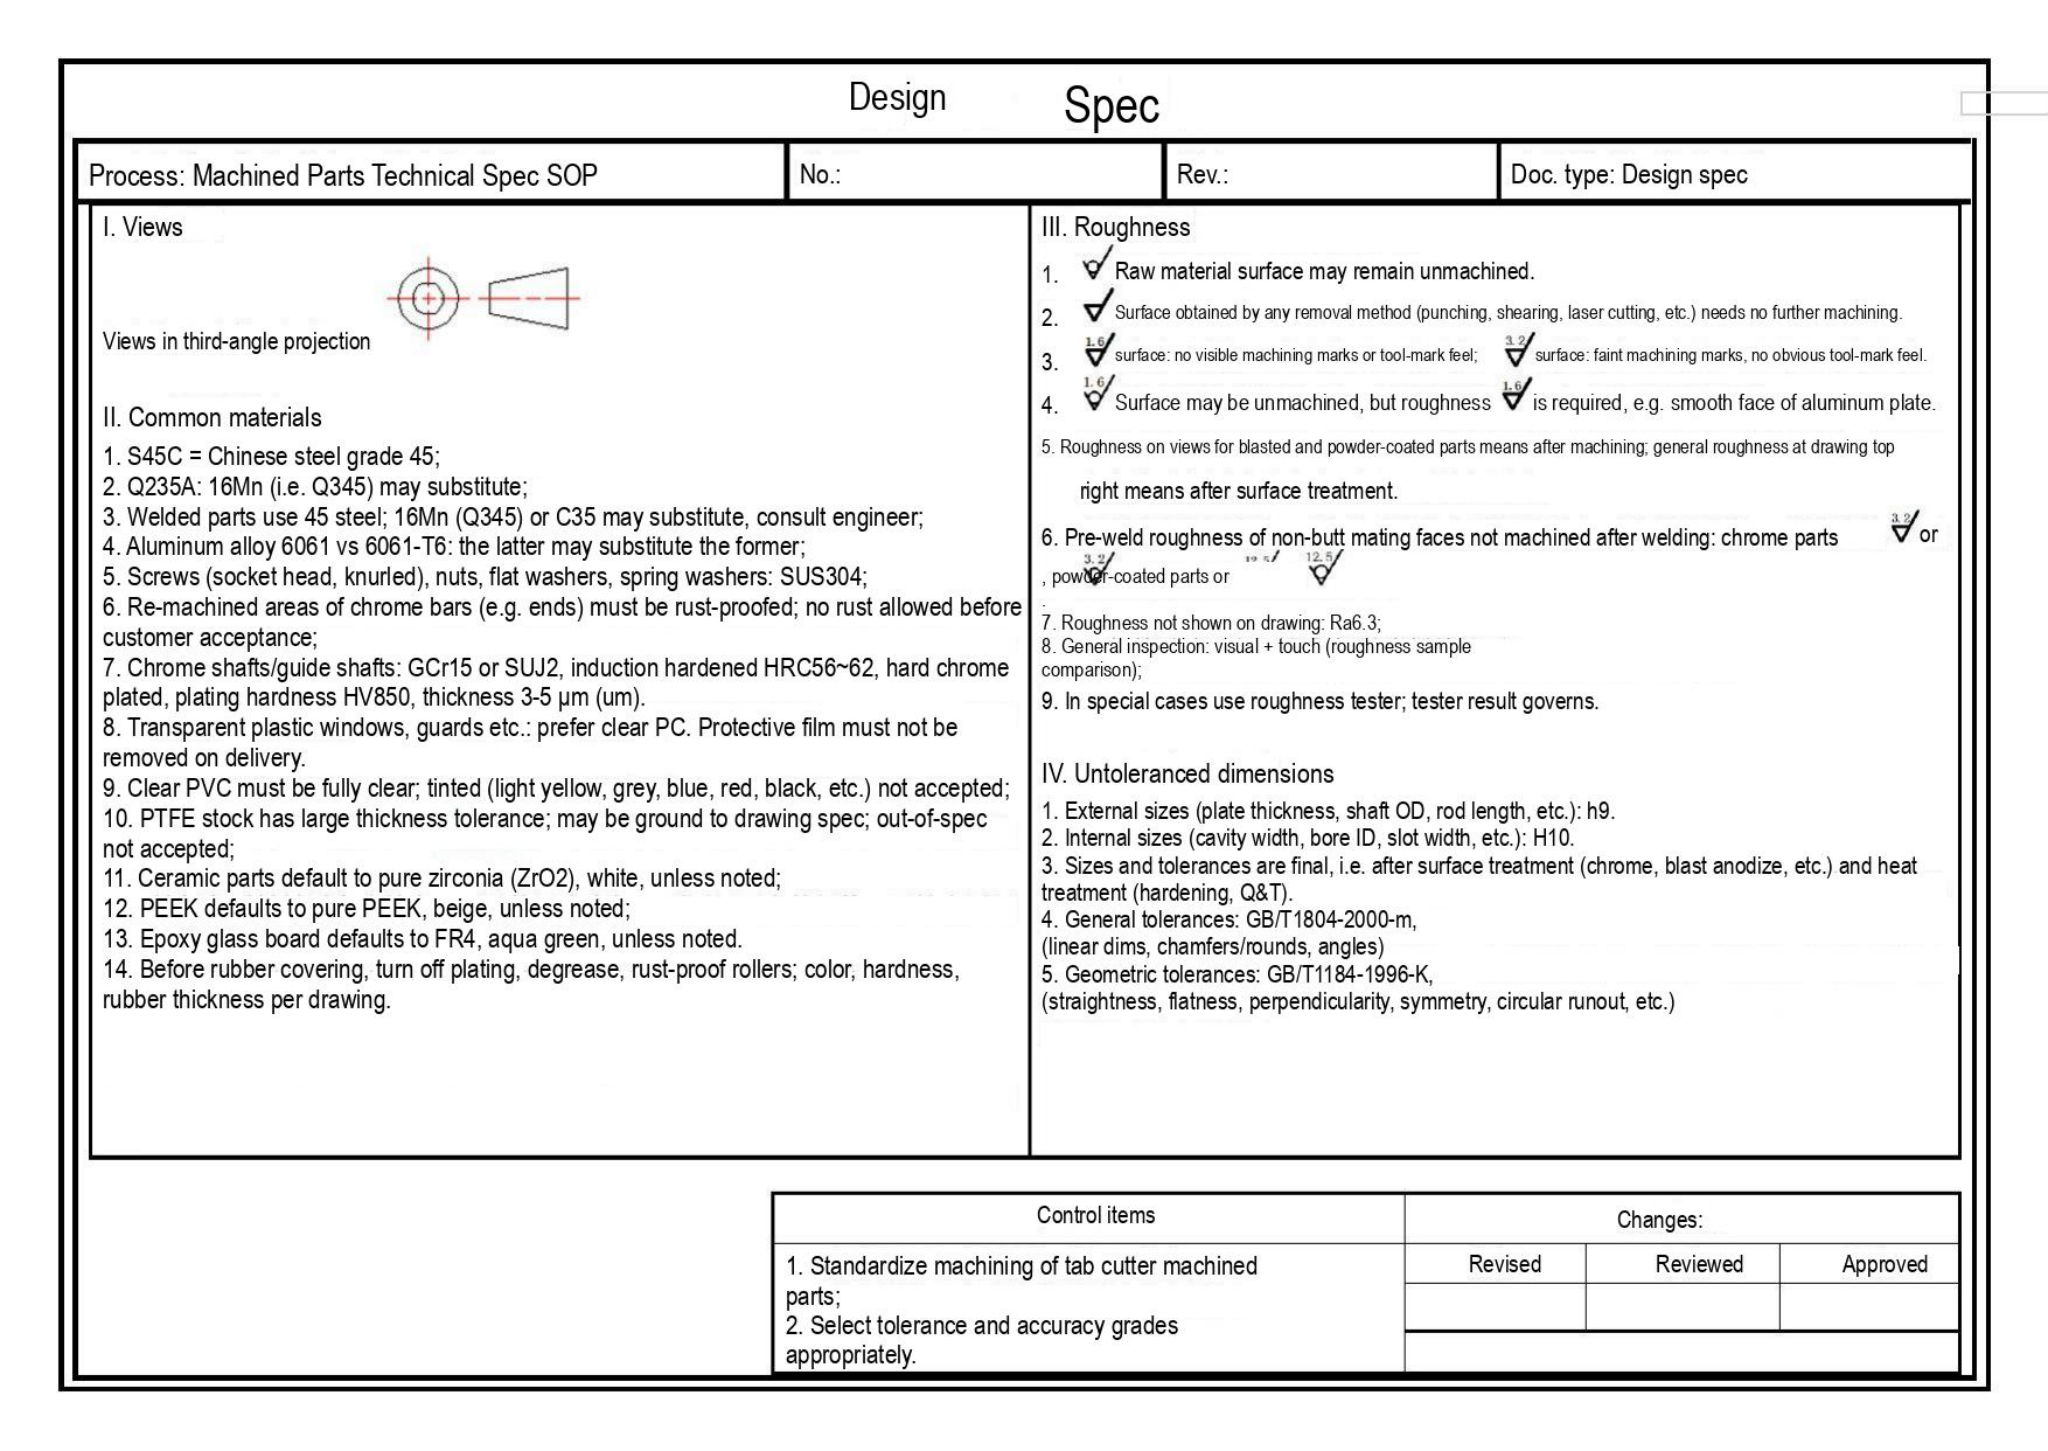Design Spec

| Process: Machined Parts Technical Spec SOP | No.: | Rev.: | Doc. type: Design spec |
|---|---|---|---|

I. Views

Views in third-angle projection

II. Common materials

1. S45C = Chinese steel grade 45;
2. Q235A: 16Mn (i.e. Q345) may substitute;
3. Welded parts use 45 steel; 16Mn (Q345) or C35 may substitute, consult engineer;
4. Aluminum alloy 6061 vs 6061-T6: the latter may substitute the former;
5. Screws (socket head, knurled), nuts, flat washers, spring washers: SUS304;
6. Re-machined areas of chrome bars (e.g. ends) must be rust-proofed; no rust allowed before customer acceptance;
7. Chrome shafts/guide shafts: GCr15 or SUJ2, induction hardened HRC56~62, hard chrome plated, plating hardness HV850, thickness 3-5 μm (um).
8. Transparent plastic windows, guards etc.: prefer clear PC. Protective film must not be removed on delivery.
9. Clear PVC must be fully clear; tinted (light yellow, grey, blue, red, black, etc.) not accepted;
10. PTFE stock has large thickness tolerance; may be ground to drawing spec; out-of-spec not accepted;
11. Ceramic parts default to pure zirconia (ZrO2), white, unless noted;
12. PEEK defaults to pure PEEK, beige, unless noted;
13. Epoxy glass board defaults to FR4, aqua green, unless noted.
14. Before rubber covering, turn off plating, degrease, rust-proof rollers; color, hardness, rubber thickness per drawing.

III. Roughness

1. Raw material surface may remain unmachined.
2. Surface obtained by any removal method (punching, shearing, laser cutting, etc.) needs no further machining.
3. 1.6 surface: no visible machining marks or tool-mark feel; 3.2 surface: faint machining marks, no obvious tool-mark feel.
4. 1.6 Surface may be unmachined, but roughness 1.6 is required, e.g. smooth face of aluminum plate.
5. Roughness on views for blasted and powder-coated parts means after machining; general roughness at drawing top right means after surface treatment.
6. Pre-weld roughness of non-butt mating faces not machined after welding: chrome parts 3.2 or 3.2, powder-coated parts or 12.5
7. Roughness not shown on drawing: Ra6.3;
8. General inspection: visual + touch (roughness sample comparison);
9. In special cases use roughness tester; tester result governs.

IV. Untoleranced dimensions

1. External sizes (plate thickness, shaft OD, rod length, etc.): h9.
2. Internal sizes (cavity width, bore ID, slot width, etc.): H10.
3. Sizes and tolerances are final, i.e. after surface treatment (chrome, blast anodize, etc.) and heat treatment (hardening, Q&T).
4. General tolerances: GB/T1804-2000-m, (linear dims, chamfers/rounds, angles)
5. Geometric tolerances: GB/T1184-1996-K, (straightness, flatness, perpendicularity, symmetry, circular runout, etc.)

| Control items | Changes: | | |
|---|---|---|---|
| 1. Standardize machining of tab cutter machined parts;<br>2. Select tolerance and accuracy grades appropriately. | Revised | Reviewed | Approved |
| | | | |
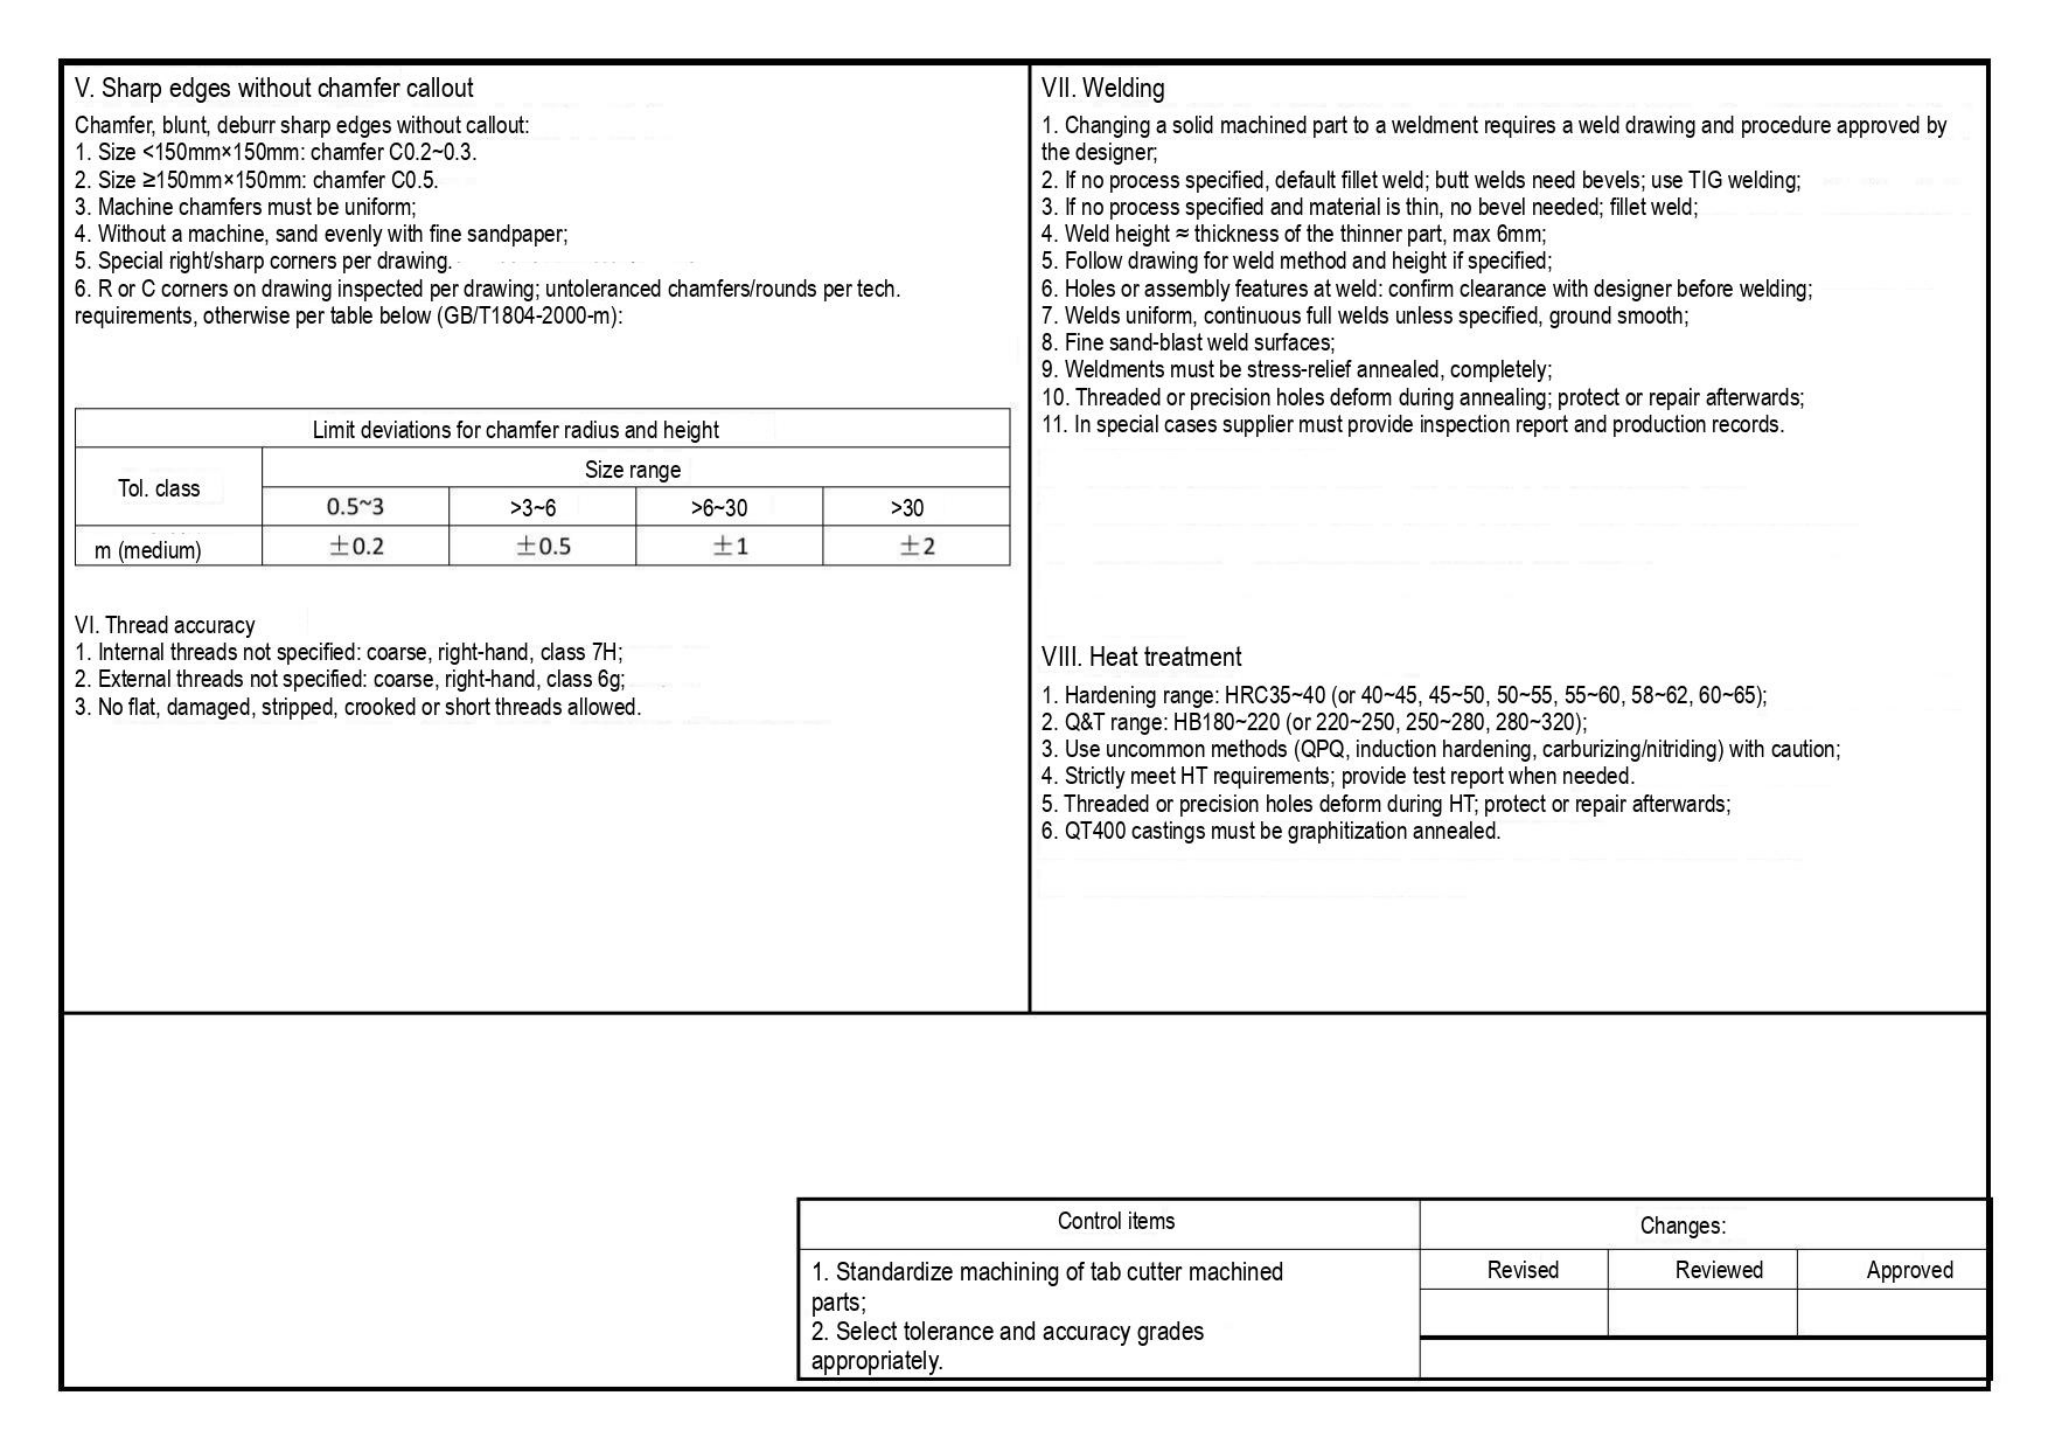V. Sharp edges without chamfer callout

Chamfer, blunt, deburr sharp edges without callout:
1. Size <150mm×150mm: chamfer C0.2~0.3.
2. Size ≥150mm×150mm: chamfer C0.5.
3. Machine chamfers must be uniform;
4. Without a machine, sand evenly with fine sandpaper;
5. Special right/sharp corners per drawing.
6. R or C corners on drawing inspected per drawing; untoleranced chamfers/rounds per tech. requirements, otherwise per table below (GB/T1804-2000-m):

Limit deviations for chamfer radius and height

| Tol. class | Size range | | | |
|---|---|---|---|---|
| | 0.5~3 | >3~6 | >6~30 | >30 |
| m (medium) | ±0.2 | ±0.5 | ±1 | ±2 |

VI. Thread accuracy
1. Internal threads not specified: coarse, right-hand, class 7H;
2. External threads not specified: coarse, right-hand, class 6g;
3. No flat, damaged, stripped, crooked or short threads allowed.

VII. Welding
1. Changing a solid machined part to a weldment requires a weld drawing and procedure approved by the designer;
2. If no process specified, default fillet weld; butt welds need bevels; use TIG welding;
3. If no process specified and material is thin, no bevel needed; fillet weld;
4. Weld height ≈ thickness of the thinner part, max 6mm;
5. Follow drawing for weld method and height if specified;
6. Holes or assembly features at weld: confirm clearance with designer before welding;
7. Welds uniform, continuous full welds unless specified, ground smooth;
8. Fine sand-blast weld surfaces;
9. Weldments must be stress-relief annealed, completely;
10. Threaded or precision holes deform during annealing; protect or repair afterwards;
11. In special cases supplier must provide inspection report and production records.

VIII. Heat treatment
1. Hardening range: HRC35~40 (or 40~45, 45~50, 50~55, 55~60, 58~62, 60~65);
2. Q&T range: HB180~220 (or 220~250, 250~280, 280~320);
3. Use uncommon methods (QPQ, induction hardening, carburizing/nitriding) with caution;
4. Strictly meet HT requirements; provide test report when needed.
5. Threaded or precision holes deform during HT; protect or repair afterwards;
6. QT400 castings must be graphitization annealed.

| Control items | Changes: | | |
|---|---|---|---|
| 1. Standardize machining of tab cutter machined parts;<br>2. Select tolerance and accuracy grades appropriately. | Revised | Reviewed | Approved |
| | | | |
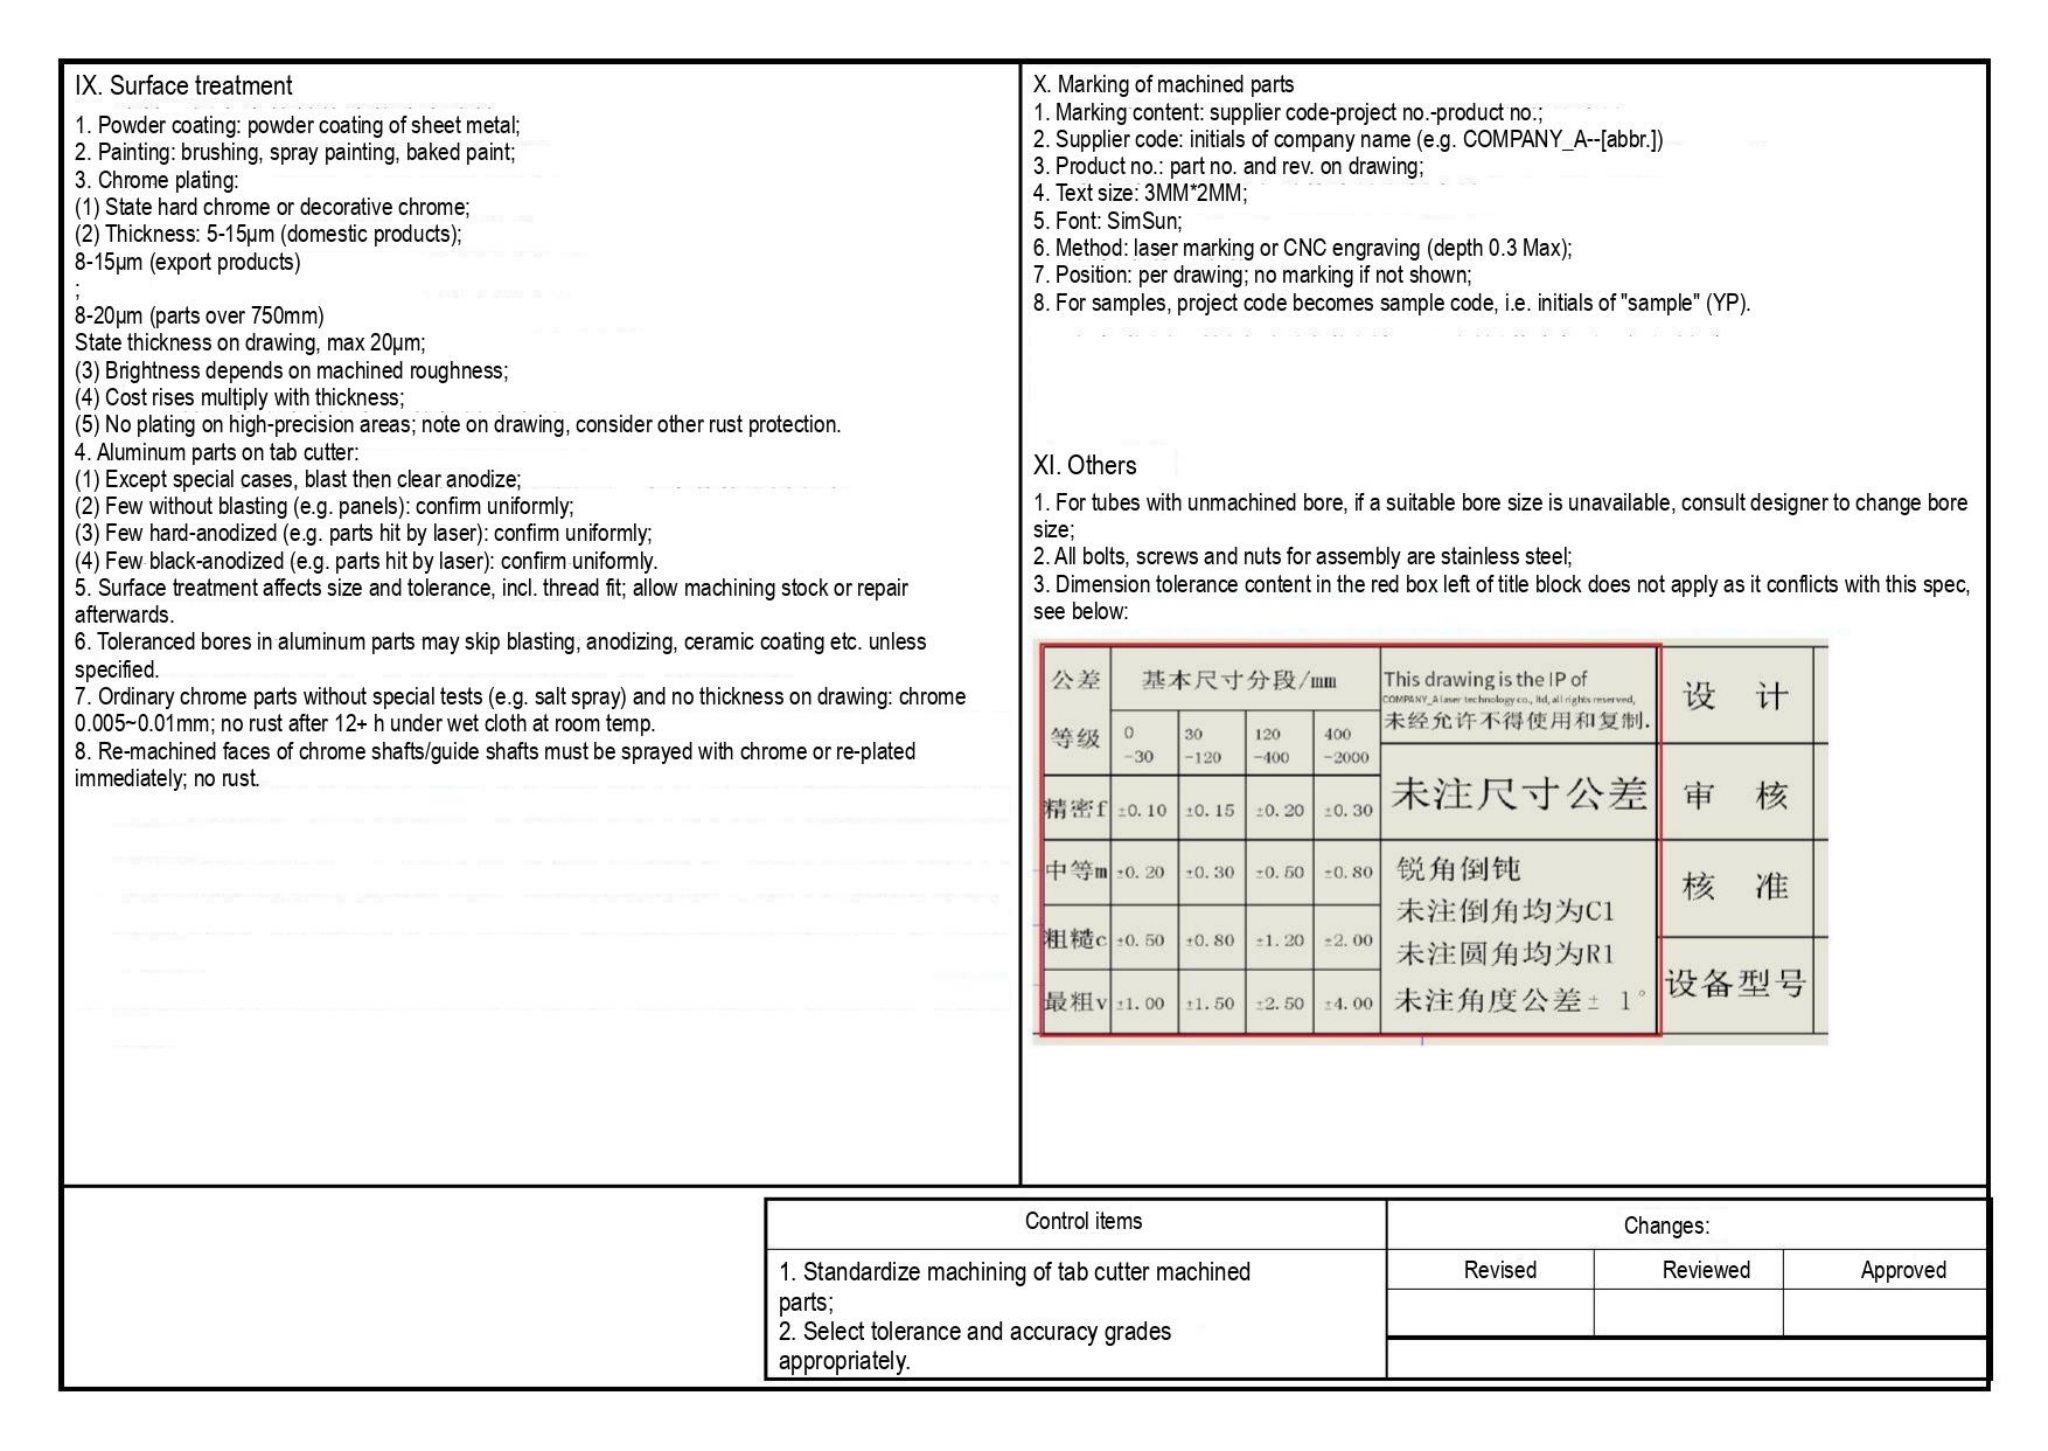IX. Surface treatment
1. Powder coating: powder coating of sheet metal;
2. Painting: brushing, spray painting, baked paint;
3. Chrome plating:
(1) State hard chrome or decorative chrome;
(2) Thickness: 5-15μm (domestic products);
8-15μm (export products)
;
8-20μm (parts over 750mm)
State thickness on drawing, max 20μm;
(3) Brightness depends on machined roughness;
(4) Cost rises multiply with thickness;
(5) No plating on high-precision areas; note on drawing, consider other rust protection.
4. Aluminum parts on tab cutter:
(1) Except special cases, blast then clear anodize;
(2) Few without blasting (e.g. panels): confirm uniformly;
(3) Few hard-anodized (e.g. parts hit by laser): confirm uniformly;
(4) Few black-anodized (e.g. parts hit by laser): confirm uniformly.
5. Surface treatment affects size and tolerance, incl. thread fit; allow machining stock or repair afterwards.
6. Toleranced bores in aluminum parts may skip blasting, anodizing, ceramic coating etc. unless specified.
7. Ordinary chrome parts without special tests (e.g. salt spray) and no thickness on drawing: chrome 0.005~0.01mm; no rust after 12+ h under wet cloth at room temp.
8. Re-machined faces of chrome shafts/guide shafts must be sprayed with chrome or re-plated immediately; no rust.

X. Marking of machined parts
1. Marking content: supplier code-project no.-product no.;
2. Supplier code: initials of company name (e.g. COMPANY_A--[abbr.])
3. Product no.: part no. and rev. on drawing;
4. Text size: 3MM*2MM;
5. Font: SimSun;
6. Method: laser marking or CNC engraving (depth 0.3 Max);
7. Position: per drawing; no marking if not shown;
8. For samples, project code becomes sample code, i.e. initials of "sample" (YP).

XI. Others
1. For tubes with unmachined bore, if a suitable bore size is unavailable, consult designer to change bore size;
2. All bolts, screws and nuts for assembly are stainless steel;
3. Dimension tolerance content in the red box left of title block does not apply as it conflicts with this spec, see below:

| 公差 等级 | 基本尺寸分段/mm 0-30 | 30-120 | 120-400 | 400-2000 | This drawing is the IP of COMPANY_A laser technology co., ltd, all rights reserved, 未经允许不得使用和复制. | 设 计 |
|---|---|---|---|---|---|---|
| 精密f | ±0.10 | ±0.15 | ±0.20 | ±0.30 | 未注尺寸公差 | 审 核 |
| 中等m | ±0.20 | ±0.30 | ±0.50 | ±0.80 | 锐角倒钝 | 核 准 |
| 粗糙c | ±0.50 | ±0.80 | ±1.20 | ±2.00 | 未注倒角均为C1 未注圆角均为R1 | |
| 最粗v | ±1.00 | ±1.50 | ±2.50 | ±4.00 | 未注角度公差± 1° | 设备型号 |

| Control items | Changes: | | |
|---|---|---|---|
| 1. Standardize machining of tab cutter machined parts; 2. Select tolerance and accuracy grades appropriately. | Revised | Reviewed | Approved |
| | | | |